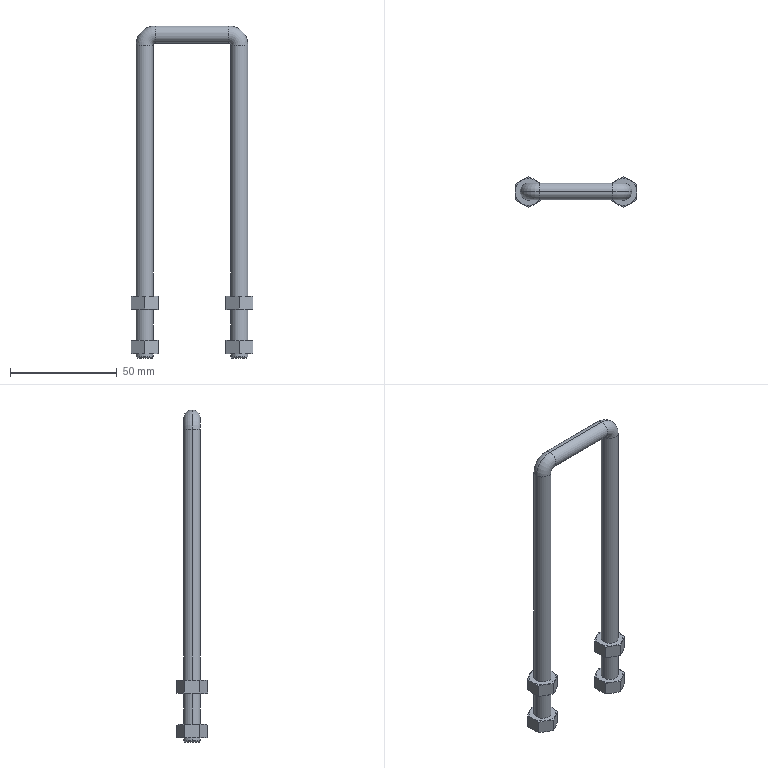Part | STEP file | _3-QC-408710.step | 1 solid | 104 faces | box 57.17 x 14.63 x 155.83 mm | volume 19518 mm3 | cone 52 | plane 34 | cylinder 14 | torus 4 | commonest cylinder face diameters 8 x14